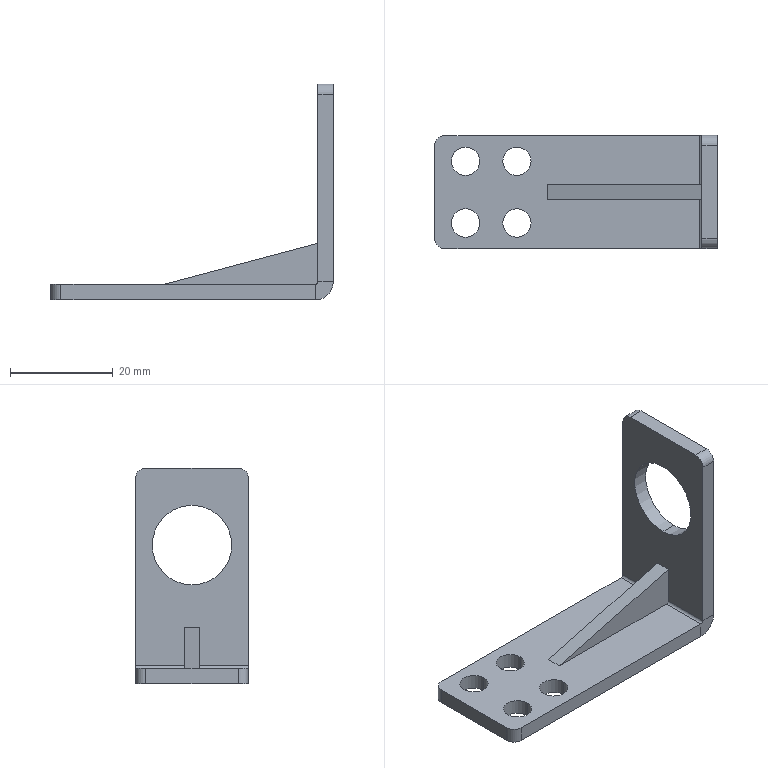Part | SolidWorks | features EdgeFlange 1, Fillet 1, FlatPattern 1, Gusset 1, HoleWzd 1, ICE 1, LPattern 1, SMBaseFlange 1, SheetMetal 1 | 2 solids | 33 faces | box 55 x 22 x 42 mm | volume 5646 mm3 | plane 17 | cylinder 16 | commonest cylinder face diameters 5.5 x8 4 x4 15.5 x2 1 x1 7 x1
STEP:
#1=CARTESIAN_POINT('',(24.5,1.5,8.));
#2=VERTEX_POINT('',#1);
#3=CARTESIAN_POINT('',(-5.5,1.5,0.));
#4=VERTEX_POINT('',#3);
#5=CARTESIAN_POINT('',(24.5,1.5,8.));
#6=DIRECTION('',(-0.9662,0.,-0.2577));
#7=VECTOR('',#6,1000.);
#8=LINE('',#5,#7);
#9=EDGE_CURVE('',#2,#4,#8,.T.);
#10=ORIENTED_EDGE('',*,*,#9,.T.);
#11=CARTESIAN_POINT('',(-5.5,-1.5,0.));
#12=VERTEX_POINT('',#11);
#13=CARTESIAN_POINT('',(-5.5,-1.5,0.));
#14=DIRECTION('',(0.,1.,0.));
#15=VECTOR('',#14,1000.);
#16=LINE('',#13,#15);
#17=EDGE_CURVE('',#12,#4,#16,.T.);
#18=ORIENTED_EDGE('',*,*,#17,.F.);
#19=CARTESIAN_POINT('',(24.5,-1.5,8.));
#20=VERTEX_POINT('',#19);
#21=CARTESIAN_POINT('',(24.5,-1.5,8.));
#22=DIRECTION('',(-0.9662,0.,-0.2577));
#23=VECTOR('',#22,1000.);
#24=LINE('',#21,#23);
#25=EDGE_CURVE('',#20,#12,#24,.T.);
#26=ORIENTED_EDGE('',*,*,#25,.F.);
#27=CARTESIAN_POINT('',(24.5,-1.5,8.));
#28=DIRECTION('',(0.,1.,0.));
#29=VECTOR('',#28,1000.);
#30=LINE('',#27,#29);
#31=EDGE_CURVE('',#20,#2,#30,.T.);
#32=ORIENTED_EDGE('',*,*,#31,.T.);
#33=EDGE_LOOP('',(#10,#18,#26,#32));
#34=FACE_OUTER_BOUND('',#33,.T.);
#35=CARTESIAN_POINT('',(24.5,-1.5,8.));
#36=DIRECTION('',(0.2577,0.,-0.9662));
#37=DIRECTION('',(-0.9662,0.,-0.2577));
#38=AXIS2_PLACEMENT_3D('',#35,#36,#37);
#39=PLANE('',#38);
#40=ADVANCED_FACE('',(#34),#39,.F.);
#41=CARTESIAN_POINT('',(24.5,1.5,0.));
#42=VERTEX_POINT('',#41);
#43=CARTESIAN_POINT('',(24.5,1.5,0.));
#44=DIRECTION('',(1.,0.,0.));
#45=VECTOR('',#44,1000.);
#46=LINE('',#43,#45);
#47=EDGE_CURVE('',#4,#42,#46,.T.);
#48=ORIENTED_EDGE('',*,*,#47,.T.);
#49=CARTESIAN_POINT('',(24.5,-1.5,0.));
#50=VERTEX_POINT('',#49);
#51=CARTESIAN_POINT('',(24.5,-1.5,0.));
#52=DIRECTION('',(0.,1.,0.));
#53=VECTOR('',#52,1000.);
#54=LINE('',#51,#53);
#55=EDGE_CURVE('',#50,#42,#54,.T.);
#56=ORIENTED_EDGE('',*,*,#55,.F.);
#57=CARTESIAN_POINT('',(24.5,-1.5,0.));
#58=DIRECTION('',(1.,0.,0.));
#59=VECTOR('',#58,1000.);
#60=LINE('',#57,#59);
#61=EDGE_CURVE('',#12,#50,#60,.T.);
#62=ORIENTED_EDGE('',*,*,#61,.F.);
#63=ORIENTED_EDGE('',*,*,#17,.T.);
#64=EDGE_LOOP('',(#48,#56,#62,#63));
#65=FACE_OUTER_BOUND('',#64,.T.);
#66=CARTESIAN_POINT('',(24.5,-1.5,0.));
#67=DIRECTION('',(0.,0.,1.));
#68=DIRECTION('',(1.,0.,0.));
#69=AXIS2_PLACEMENT_3D('',#66,#67,#68);
#70=PLANE('',#69);
#71=ADVANCED_FACE('',(#65),#70,.F.);
#72=CARTESIAN_POINT('',(24.5,1.5,0.));
#73=DIRECTION('',(0.,0.,1.));
#74=VECTOR('',#73,1000.);
#75=LINE('',#72,#74);
#76=EDGE_CURVE('',#42,#2,#75,.T.);
#77=ORIENTED_EDGE('',*,*,#76,.T.);
#78=ORIENTED_EDGE('',*,*,#31,.F.);
#79=CARTESIAN_POINT('',(24.5,-1.5,0.));
#80=DIRECTION('',(0.,0.,1.));
#81=VECTOR('',#80,1000.);
#82=LINE('',#79,#81);
#83=EDGE_CURVE('',#50,#20,#82,.T.);
#84=ORIENTED_EDGE('',*,*,#83,.F.);
#85=ORIENTED_EDGE('',*,*,#55,.T.);
#86=EDGE_LOOP('',(#77,#78,#84,#85));
#87=FACE_OUTER_BOUND('',#86,.T.);
#88=CARTESIAN_POINT('',(24.5,-1.5,0.));
#89=DIRECTION('',(-1.,0.,0.));
#90=DIRECTION('',(0.,0.,1.));
#91=AXIS2_PLACEMENT_3D('',#88,#89,#90);
#92=PLANE('',#91);
#93=ADVANCED_FACE('',(#87),#92,.F.);
#94=ORIENTED_EDGE('',*,*,#25,.T.);
#95=ORIENTED_EDGE('',*,*,#61,.T.);
#96=ORIENTED_EDGE('',*,*,#83,.T.);
#97=EDGE_LOOP('',(#94,#95,#96));
#98=FACE_OUTER_BOUND('',#97,.T.);
#99=CARTESIAN_POINT('',(0.,-1.5,0.));
#100=DIRECTION('',(0.,1.,0.));
#101=DIRECTION('',(0.,0.,1.));
#102=AXIS2_PLACEMENT_3D('',#99,#100,#101);
#103=PLANE('',#102);
#104=ADVANCED_FACE('',(#98),#103,.F.);
#105=ORIENTED_EDGE('',*,*,#9,.F.);
#106=ORIENTED_EDGE('',*,*,#76,.F.);
#107=ORIENTED_EDGE('',*,*,#47,.F.);
#108=EDGE_LOOP('',(#105,#106,#107));
#109=FACE_OUTER_BOUND('',#108,.T.);
#110=CARTESIAN_POINT('',(0.,1.5,0.));
#111=DIRECTION('',(0.,1.,0.));
#112=DIRECTION('',(0.,0.,1.));
#113=AXIS2_PLACEMENT_3D('',#110,#111,#112);
#114=PLANE('',#113);
#115=ADVANCED_FACE('',(#109),#114,.T.);
#116=CLOSED_SHELL('',(#40,#71,#93,#104,#115));
#117=MANIFOLD_SOLID_BREP('',#116);
#118=CARTESIAN_POINT('',(-14.25,6.,-3.));
#119=VERTEX_POINT('',#118);
#120=CARTESIAN_POINT('',(-8.75,6.,-3.));
#121=VERTEX_POINT('',#120);
#122=CARTESIAN_POINT('',(-11.5,6.,-3.));
#123=DIRECTION('',(0.,0.,1.));
#124=DIRECTION('',(1.,0.,0.));
#125=AXIS2_PLACEMENT_3D('',#122,#123,#124);
#126=CIRCLE('',#125,2.75);
#127=EDGE_CURVE('',#119,#121,#126,.T.);
#128=ORIENTED_EDGE('',*,*,#127,.F.);
#129=CARTESIAN_POINT('',(-14.25,6.,0.));
#130=VERTEX_POINT('',#129);
#131=CARTESIAN_POINT('',(-14.25,6.,0.));
#132=DIRECTION('',(0.,0.,1.));
#133=VECTOR('',#132,1000.);
#134=LINE('',#131,#133);
#135=EDGE_CURVE('',#119,#130,#134,.T.);
#136=ORIENTED_EDGE('',*,*,#135,.T.);
#137=CARTESIAN_POINT('',(-8.75,6.,0.));
#138=VERTEX_POINT('',#137);
#139=CARTESIAN_POINT('',(-11.5,6.,0.));
#140=DIRECTION('',(0.,0.,1.));
#141=DIRECTION('',(1.,0.,0.));
#142=AXIS2_PLACEMENT_3D('',#139,#140,#141);
#143=CIRCLE('',#142,2.75);
#144=EDGE_CURVE('',#130,#138,#143,.T.);
#145=ORIENTED_EDGE('',*,*,#144,.T.);
#146=CARTESIAN_POINT('',(-8.75,6.,0.));
#147=DIRECTION('',(0.,0.,1.));
#148=VECTOR('',#147,1000.);
#149=LINE('',#146,#148);
#150=EDGE_CURVE('',#121,#138,#149,.T.);
#151=ORIENTED_EDGE('',*,*,#150,.F.);
#152=EDGE_LOOP('',(#128,#136,#145,#151));
#153=FACE_OUTER_BOUND('',#152,.T.);
#154=CARTESIAN_POINT('',(-11.5,6.,0.));
#155=DIRECTION('',(0.,0.,1.));
#156=DIRECTION('',(1.,0.,0.));
#157=AXIS2_PLACEMENT_3D('',#154,#155,#156);
#158=CYLINDRICAL_SURFACE('',#157,2.75);
#159=ADVANCED_FACE('',(#153),#158,.F.);
#160=CARTESIAN_POINT('',(-14.25,-6.,-3.));
#161=VERTEX_POINT('',#160);
#162=CARTESIAN_POINT('',(-8.75,-6.,-3.));
#163=VERTEX_POINT('',#162);
#164=CARTESIAN_POINT('',(-11.5,-6.,-3.));
#165=DIRECTION('',(0.,0.,1.));
#166=DIRECTION('',(1.,0.,0.));
#167=AXIS2_PLACEMENT_3D('',#164,#165,#166);
#168=CIRCLE('',#167,2.75);
#169=EDGE_CURVE('',#161,#163,#168,.T.);
#170=ORIENTED_EDGE('',*,*,#169,.F.);
#171=CARTESIAN_POINT('',(-14.25,-6.,0.));
#172=VERTEX_POINT('',#171);
#173=CARTESIAN_POINT('',(-14.25,-6.,0.));
#174=DIRECTION('',(0.,0.,1.));
#175=VECTOR('',#174,1000.);
#176=LINE('',#173,#175);
#177=EDGE_CURVE('',#161,#172,#176,.T.);
#178=ORIENTED_EDGE('',*,*,#177,.T.);
#179=CARTESIAN_POINT('',(-8.75,-6.,0.));
#180=VERTEX_POINT('',#179);
#181=CARTESIAN_POINT('',(-11.5,-6.,0.));
#182=DIRECTION('',(0.,0.,1.));
#183=DIRECTION('',(1.,0.,0.));
#184=AXIS2_PLACEMENT_3D('',#181,#182,#183);
#185=CIRCLE('',#184,2.75);
#186=EDGE_CURVE('',#172,#180,#185,.T.);
#187=ORIENTED_EDGE('',*,*,#186,.T.);
#188=CARTESIAN_POINT('',(-8.75,-6.,0.));
#189=DIRECTION('',(0.,0.,1.));
#190=VECTOR('',#189,1000.);
#191=LINE('',#188,#190);
#192=EDGE_CURVE('',#163,#180,#191,.T.);
#193=ORIENTED_EDGE('',*,*,#192,.F.);
#194=EDGE_LOOP('',(#170,#178,#187,#193));
#195=FACE_OUTER_BOUND('',#194,.T.);
#196=CARTESIAN_POINT('',(-11.5,-6.,0.));
#197=DIRECTION('',(0.,0.,1.));
#198=DIRECTION('',(1.,0.,0.));
#199=AXIS2_PLACEMENT_3D('',#196,#197,#198);
#200=CYLINDRICAL_SURFACE('',#199,2.75);
#201=ADVANCED_FACE('',(#195),#200,.F.);
#202=CARTESIAN_POINT('',(-24.25,-6.,-3.));
#203=VERTEX_POINT('',#202);
#204=CARTESIAN_POINT('',(-18.75,-6.,-3.));
#205=VERTEX_POINT('',#204);
#206=CARTESIAN_POINT('',(-21.5,-6.,-3.));
#207=DIRECTION('',(0.,0.,1.));
#208=DIRECTION('',(1.,0.,0.));
#209=AXIS2_PLACEMENT_3D('',#206,#207,#208);
#210=CIRCLE('',#209,2.75);
#211=EDGE_CURVE('',#203,#205,#210,.T.);
#212=ORIENTED_EDGE('',*,*,#211,.F.);
#213=CARTESIAN_POINT('',(-24.25,-6.,0.));
#214=VERTEX_POINT('',#213);
#215=CARTESIAN_POINT('',(-24.25,-6.,0.));
#216=DIRECTION('',(0.,0.,1.));
#217=VECTOR('',#216,1000.);
#218=LINE('',#215,#217);
#219=EDGE_CURVE('',#203,#214,#218,.T.);
#220=ORIENTED_EDGE('',*,*,#219,.T.);
#221=CARTESIAN_POINT('',(-18.75,-6.,0.));
#222=VERTEX_POINT('',#221);
#223=CARTESIAN_POINT('',(-21.5,-6.,0.));
#224=DIRECTION('',(0.,0.,1.));
#225=DIRECTION('',(1.,0.,0.));
#226=AXIS2_PLACEMENT_3D('',#223,#224,#225);
#227=CIRCLE('',#226,2.75);
#228=EDGE_CURVE('',#214,#222,#227,.T.);
#229=ORIENTED_EDGE('',*,*,#228,.T.);
#230=CARTESIAN_POINT('',(-18.75,-6.,0.));
#231=DIRECTION('',(0.,0.,1.));
#232=VECTOR('',#231,1000.);
#233=LINE('',#230,#232);
#234=EDGE_CURVE('',#205,#222,#233,.T.);
#235=ORIENTED_EDGE('',*,*,#234,.F.);
#236=EDGE_LOOP('',(#212,#220,#229,#235));
#237=FACE_OUTER_BOUND('',#236,.T.);
#238=CARTESIAN_POINT('',(-21.5,-6.,0.));
#239=DIRECTION('',(0.,0.,1.));
#240=DIRECTION('',(1.,0.,0.));
#241=AXIS2_PLACEMENT_3D('',#238,#239,#240);
#242=CYLINDRICAL_SURFACE('',#241,2.75);
#243=ADVANCED_FACE('',(#237),#242,.F.);
#244=CARTESIAN_POINT('',(-24.25,6.,-3.));
#245=VERTEX_POINT('',#244);
#246=CARTESIAN_POINT('',(-18.75,6.,-3.));
#247=VERTEX_POINT('',#246);
#248=CARTESIAN_POINT('',(-21.5,6.,-3.));
#249=DIRECTION('',(0.,0.,1.));
#250=DIRECTION('',(1.,0.,0.));
#251=AXIS2_PLACEMENT_3D('',#248,#249,#250);
#252=CIRCLE('',#251,2.75);
#253=EDGE_CURVE('',#245,#247,#252,.T.);
#254=ORIENTED_EDGE('',*,*,#253,.F.);
#255=CARTESIAN_POINT('',(-24.25,6.,0.));
#256=VERTEX_POINT('',#255);
#257=CARTESIAN_POINT('',(-24.25,6.,0.));
#258=DIRECTION('',(0.,0.,1.));
#259=VECTOR('',#258,1000.);
#260=LINE('',#257,#259);
#261=EDGE_CURVE('',#245,#256,#260,.T.);
#262=ORIENTED_EDGE('',*,*,#261,.T.);
#263=CARTESIAN_POINT('',(-18.75,6.,0.));
#264=VERTEX_POINT('',#263);
#265=CARTESIAN_POINT('',(-21.5,6.,0.));
#266=DIRECTION('',(0.,0.,1.));
#267=DIRECTION('',(1.,0.,0.));
#268=AXIS2_PLACEMENT_3D('',#265,#266,#267);
#269=CIRCLE('',#268,2.75);
#270=EDGE_CURVE('',#256,#264,#269,.T.);
#271=ORIENTED_EDGE('',*,*,#270,.T.);
#272=CARTESIAN_POINT('',(-18.75,6.,0.));
#273=DIRECTION('',(0.,0.,1.));
#274=VECTOR('',#273,1000.);
#275=LINE('',#272,#274);
#276=EDGE_CURVE('',#247,#264,#275,.T.);
#277=ORIENTED_EDGE('',*,*,#276,.F.);
#278=EDGE_LOOP('',(#254,#262,#271,#277));
#279=FACE_OUTER_BOUND('',#278,.T.);
#280=CARTESIAN_POINT('',(-21.5,6.,0.));
#281=DIRECTION('',(0.,0.,1.));
#282=DIRECTION('',(1.,0.,0.));
#283=AXIS2_PLACEMENT_3D('',#280,#281,#282);
#284=CYLINDRICAL_SURFACE('',#283,2.75);
#285=ADVANCED_FACE('',(#279),#284,.F.);
#286=CARTESIAN_POINT('',(27.5,0.,31.75));
#287=VERTEX_POINT('',#286);
#288=CARTESIAN_POINT('',(27.5,0.,16.25));
#289=VERTEX_POINT('',#288);
#290=CARTESIAN_POINT('',(27.5,0.,24.));
#291=DIRECTION('',(1.,0.,0.));
#292=DIRECTION('',(0.,0.,1.));
#293=AXIS2_PLACEMENT_3D('',#290,#291,#292);
#294=CIRCLE('',#293,7.75);
#295=EDGE_CURVE('',#287,#289,#294,.T.);
#296=ORIENTED_EDGE('',*,*,#295,.T.);
#297=CARTESIAN_POINT('',(24.5,0.,16.25));
#298=VERTEX_POINT('',#297);
#299=CARTESIAN_POINT('',(27.501,0.,16.25));
#300=DIRECTION('',(-1.,0.,0.));
#301=VECTOR('',#300,1000.);
#302=LINE('',#299,#301);
#303=EDGE_CURVE('',#289,#298,#302,.T.);
#304=ORIENTED_EDGE('',*,*,#303,.T.);
#305=CARTESIAN_POINT('',(24.5,0.,31.75));
#306=VERTEX_POINT('',#305);
#307=CARTESIAN_POINT('',(24.5,0.,24.));
#308=DIRECTION('',(-1.,0.,0.));
#309=DIRECTION('',(0.,0.,1.));
#310=AXIS2_PLACEMENT_3D('',#307,#308,#309);
#311=CIRCLE('',#310,7.75);
#312=EDGE_CURVE('',#298,#306,#311,.T.);
#313=ORIENTED_EDGE('',*,*,#312,.T.);
#314=CARTESIAN_POINT('',(27.501,0.,31.75));
#315=DIRECTION('',(-1.,0.,0.));
#316=VECTOR('',#315,1000.);
#317=LINE('',#314,#316);
#318=EDGE_CURVE('',#287,#306,#317,.T.);
#319=ORIENTED_EDGE('',*,*,#318,.F.);
#320=EDGE_LOOP('',(#296,#304,#313,#319));
#321=FACE_OUTER_BOUND('',#320,.T.);
#322=CARTESIAN_POINT('',(27.501,0.,24.));
#323=DIRECTION('',(-1.,0.,0.));
#324=DIRECTION('',(0.,0.,1.));
#325=AXIS2_PLACEMENT_3D('',#322,#323,#324);
#326=CYLINDRICAL_SURFACE('',#325,7.75);
#327=ADVANCED_FACE('',(#321),#326,.F.);
#328=CARTESIAN_POINT('',(24.,11.,-3.));
#329=VERTEX_POINT('',#328);
#330=CARTESIAN_POINT('',(-25.5,11.,-3.));
#331=VERTEX_POINT('',#330);
#332=CARTESIAN_POINT('',(27.5,11.,-3.));
#333=DIRECTION('',(-1.,0.,0.));
#334=VECTOR('',#333,1000.);
#335=LINE('',#332,#334);
#336=EDGE_CURVE('',#329,#331,#335,.T.);
#337=ORIENTED_EDGE('',*,*,#336,.T.);
#338=CARTESIAN_POINT('',(-25.5,11.,0.));
#339=VERTEX_POINT('',#338);
#340=CARTESIAN_POINT('',(-25.5,11.,-3.));
#341=DIRECTION('',(0.,0.,1.));
#342=VECTOR('',#341,1000.);
#343=LINE('',#340,#342);
#344=EDGE_CURVE('',#331,#339,#343,.T.);
#345=ORIENTED_EDGE('',*,*,#344,.T.);
#346=CARTESIAN_POINT('',(24.,11.,0.));
#347=VERTEX_POINT('',#346);
#348=CARTESIAN_POINT('',(27.5,11.,0.));
#349=DIRECTION('',(-1.,0.,0.));
#350=VECTOR('',#349,1000.);
#351=LINE('',#348,#350);
#352=EDGE_CURVE('',#347,#339,#351,.T.);
#353=ORIENTED_EDGE('',*,*,#352,.F.);
#354=CARTESIAN_POINT('',(24.,11.,0.));
#355=DIRECTION('',(0.,0.,-1.));
#356=VECTOR('',#355,1000.);
#357=LINE('',#354,#356);
#358=EDGE_CURVE('',#347,#329,#357,.T.);
#359=ORIENTED_EDGE('',*,*,#358,.T.);
#360=EDGE_LOOP('',(#337,#345,#353,#359));
#361=FACE_OUTER_BOUND('',#360,.T.);
#362=CARTESIAN_POINT('',(27.5,11.,-3.));
#363=DIRECTION('',(0.,1.,0.));
#364=DIRECTION('',(-1.,0.,0.));
#365=AXIS2_PLACEMENT_3D('',#362,#363,#364);
#366=PLANE('',#365);
#367=ADVANCED_FACE('',(#361),#366,.T.);
#368=CARTESIAN_POINT('',(-11.5,6.,-3.));
#369=DIRECTION('',(0.,0.,1.));
#370=DIRECTION('',(1.,0.,0.));
#371=AXIS2_PLACEMENT_3D('',#368,#369,#370);
#372=CIRCLE('',#371,2.75);
#373=EDGE_CURVE('',#121,#119,#372,.T.);
#374=ORIENTED_EDGE('',*,*,#373,.T.);
#375=ORIENTED_EDGE('',*,*,#127,.T.);
#376=EDGE_LOOP('',(#374,#375));
#377=FACE_BOUND('',#376,.T.);
#378=CARTESIAN_POINT('',(-11.5,-6.,-3.));
#379=DIRECTION('',(0.,0.,1.));
#380=DIRECTION('',(1.,0.,0.));
#381=AXIS2_PLACEMENT_3D('',#378,#379,#380);
#382=CIRCLE('',#381,2.75);
#383=EDGE_CURVE('',#163,#161,#382,.T.);
#384=ORIENTED_EDGE('',*,*,#383,.T.);
#385=ORIENTED_EDGE('',*,*,#169,.T.);
#386=EDGE_LOOP('',(#384,#385));
#387=FACE_BOUND('',#386,.T.);
#388=CARTESIAN_POINT('',(-21.5,-6.,-3.));
#389=DIRECTION('',(0.,0.,1.));
#390=DIRECTION('',(1.,0.,0.));
#391=AXIS2_PLACEMENT_3D('',#388,#389,#390);
#392=CIRCLE('',#391,2.75);
#393=EDGE_CURVE('',#205,#203,#392,.T.);
#394=ORIENTED_EDGE('',*,*,#393,.T.);
#395=ORIENTED_EDGE('',*,*,#211,.T.);
#396=EDGE_LOOP('',(#394,#395));
#397=FACE_BOUND('',#396,.T.);
#398=CARTESIAN_POINT('',(-21.5,6.,-3.));
#399=DIRECTION('',(0.,0.,1.));
#400=DIRECTION('',(1.,0.,0.));
#401=AXIS2_PLACEMENT_3D('',#398,#399,#400);
#402=CIRCLE('',#401,2.75);
#403=EDGE_CURVE('',#247,#245,#402,.T.);
#404=ORIENTED_EDGE('',*,*,#403,.T.);
#405=ORIENTED_EDGE('',*,*,#253,.T.);
#406=EDGE_LOOP('',(#404,#405));
#407=FACE_BOUND('',#406,.T.);
#408=CARTESIAN_POINT('',(-27.5,9.,-3.));
#409=VERTEX_POINT('',#408);
#410=CARTESIAN_POINT('',(-27.5,-9.,-3.));
#411=VERTEX_POINT('',#410);
#412=CARTESIAN_POINT('',(-27.5,-11.,-3.));
#413=DIRECTION('',(0.,-1.,0.));
#414=VECTOR('',#413,1000.);
#415=LINE('',#412,#414);
#416=EDGE_CURVE('',#409,#411,#415,.T.);
#417=ORIENTED_EDGE('',*,*,#416,.F.);
#418=CARTESIAN_POINT('',(-25.5,9.,-3.));
#419=DIRECTION('',(0.,0.,-1.));
#420=DIRECTION('',(1.,0.,0.));
#421=AXIS2_PLACEMENT_3D('',#418,#419,#420);
#422=CIRCLE('',#421,2.);
#423=EDGE_CURVE('',#409,#331,#422,.T.);
#424=ORIENTED_EDGE('',*,*,#423,.T.);
#425=ORIENTED_EDGE('',*,*,#336,.F.);
#426=CARTESIAN_POINT('',(24.,-11.,-3.));
#427=VERTEX_POINT('',#426);
#428=CARTESIAN_POINT('',(24.,11.,-3.));
#429=DIRECTION('',(0.,-1.,0.));
#430=VECTOR('',#429,1000.);
#431=LINE('',#428,#430);
#432=EDGE_CURVE('',#329,#427,#431,.T.);
#433=ORIENTED_EDGE('',*,*,#432,.T.);
#434=CARTESIAN_POINT('',(-25.5,-11.,-3.));
#435=VERTEX_POINT('',#434);
#436=CARTESIAN_POINT('',(27.5,-11.,-3.));
#437=DIRECTION('',(1.,0.,0.));
#438=VECTOR('',#437,1000.);
#439=LINE('',#436,#438);
#440=EDGE_CURVE('',#435,#427,#439,.T.);
#441=ORIENTED_EDGE('',*,*,#440,.F.);
#442=CARTESIAN_POINT('',(-25.5,-9.,-3.));
#443=DIRECTION('',(0.,0.,-1.));
#444=DIRECTION('',(1.,0.,0.));
#445=AXIS2_PLACEMENT_3D('',#442,#443,#444);
#446=CIRCLE('',#445,2.);
#447=EDGE_CURVE('',#435,#411,#446,.T.);
#448=ORIENTED_EDGE('',*,*,#447,.T.);
#449=EDGE_LOOP('',(#417,#424,#425,#433,#441,#448));
#450=FACE_OUTER_BOUND('',#449,.T.);
#451=CARTESIAN_POINT('',(0.,0.,-3.));
#452=DIRECTION('',(0.,0.,1.));
#453=DIRECTION('',(1.,0.,0.));
#454=AXIS2_PLACEMENT_3D('',#451,#452,#453);
#455=PLANE('',#454);
#456=ADVANCED_FACE('',(#377,#387,#397,#407,#450),#455,.F.);
#457=CARTESIAN_POINT('',(-11.5,6.,0.));
#458=DIRECTION('',(0.,0.,1.));
#459=DIRECTION('',(1.,0.,0.));
#460=AXIS2_PLACEMENT_3D('',#457,#458,#459);
#461=CIRCLE('',#460,2.75);
#462=EDGE_CURVE('',#138,#130,#461,.T.);
#463=ORIENTED_EDGE('',*,*,#462,.F.);
#464=ORIENTED_EDGE('',*,*,#144,.F.);
#465=EDGE_LOOP('',(#463,#464));
#466=FACE_BOUND('',#465,.T.);
#467=CARTESIAN_POINT('',(-11.5,-6.,0.));
#468=DIRECTION('',(0.,0.,1.));
#469=DIRECTION('',(1.,0.,0.));
#470=AXIS2_PLACEMENT_3D('',#467,#468,#469);
#471=CIRCLE('',#470,2.75);
#472=EDGE_CURVE('',#180,#172,#471,.T.);
#473=ORIENTED_EDGE('',*,*,#472,.F.);
#474=ORIENTED_EDGE('',*,*,#186,.F.);
#475=EDGE_LOOP('',(#473,#474));
#476=FACE_BOUND('',#475,.T.);
#477=CARTESIAN_POINT('',(-21.5,-6.,0.));
#478=DIRECTION('',(0.,0.,1.));
#479=DIRECTION('',(1.,0.,0.));
#480=AXIS2_PLACEMENT_3D('',#477,#478,#479);
#481=CIRCLE('',#480,2.75);
#482=EDGE_CURVE('',#222,#214,#481,.T.);
#483=ORIENTED_EDGE('',*,*,#482,.F.);
#484=ORIENTED_EDGE('',*,*,#228,.F.);
#485=EDGE_LOOP('',(#483,#484));
#486=FACE_BOUND('',#485,.T.);
#487=CARTESIAN_POINT('',(-21.5,6.,0.));
#488=DIRECTION('',(0.,0.,1.));
#489=DIRECTION('',(1.,0.,0.));
#490=AXIS2_PLACEMENT_3D('',#487,#488,#489);
#491=CIRCLE('',#490,2.75);
#492=EDGE_CURVE('',#264,#256,#491,.T.);
#493=ORIENTED_EDGE('',*,*,#492,.F.);
#494=ORIENTED_EDGE('',*,*,#270,.F.);
#495=EDGE_LOOP('',(#493,#494));
#496=FACE_BOUND('',#495,.T.);
#497=ORIENTED_EDGE('',*,*,#352,.T.);
#498=CARTESIAN_POINT('',(-27.5,9.,0.));
#499=VERTEX_POINT('',#498);
#500=CARTESIAN_POINT('',(-25.5,9.,0.));
#501=DIRECTION('',(0.,0.,1.));
#502=DIRECTION('',(1.,0.,0.));
#503=AXIS2_PLACEMENT_3D('',#500,#501,#502);
#504=CIRCLE('',#503,2.);
#505=EDGE_CURVE('',#339,#499,#504,.T.);
#506=ORIENTED_EDGE('',*,*,#505,.T.);
#507=CARTESIAN_POINT('',(-27.5,-9.,0.));
#508=VERTEX_POINT('',#507);
#509=CARTESIAN_POINT('',(-27.5,-11.,0.));
#510=DIRECTION('',(0.,-1.,0.));
#511=VECTOR('',#510,1000.);
#512=LINE('',#509,#511);
#513=EDGE_CURVE('',#499,#508,#512,.T.);
#514=ORIENTED_EDGE('',*,*,#513,.T.);
#515=CARTESIAN_POINT('',(-25.5,-11.,0.));
#516=VERTEX_POINT('',#515);
#517=CARTESIAN_POINT('',(-25.5,-9.,0.));
#518=DIRECTION('',(0.,0.,1.));
#519=DIRECTION('',(1.,0.,0.));
#520=AXIS2_PLACEMENT_3D('',#517,#518,#519);
#521=CIRCLE('',#520,2.);
#522=EDGE_CURVE('',#508,#516,#521,.T.);
#523=ORIENTED_EDGE('',*,*,#522,.T.);
#524=CARTESIAN_POINT('',(24.,-11.,0.));
#525=VERTEX_POINT('',#524);
#526=CARTESIAN_POINT('',(27.5,-11.,0.));
#527=DIRECTION('',(1.,0.,0.));
#528=VECTOR('',#527,1000.);
#529=LINE('',#526,#528);
#530=EDGE_CURVE('',#516,#525,#529,.T.);
#531=ORIENTED_EDGE('',*,*,#530,.T.);
#532=CARTESIAN_POINT('',(24.,11.,0.));
#533=DIRECTION('',(0.,-1.,0.));
#534=VECTOR('',#533,1000.);
#535=LINE('',#532,#534);
#536=EDGE_CURVE('',#347,#525,#535,.T.);
#537=ORIENTED_EDGE('',*,*,#536,.F.);
#538=EDGE_LOOP('',(#497,#506,#514,#523,#531,#537));
#539=FACE_OUTER_BOUND('',#538,.T.);
#540=CARTESIAN_POINT('',(0.,0.,0.));
#541=DIRECTION('',(0.,0.,1.));
#542=DIRECTION('',(1.,0.,0.));
#543=AXIS2_PLACEMENT_3D('',#540,#541,#542);
#544=PLANE('',#543);
#545=ADVANCED_FACE('',(#466,#476,#486,#496,#539),#544,.T.);
#546=ORIENTED_EDGE('',*,*,#513,.F.);
#547=CARTESIAN_POINT('',(-27.5,9.,-3.));
#548=DIRECTION('',(0.,0.,-1.));
#549=VECTOR('',#548,1000.);
#550=LINE('',#547,#549);
#551=EDGE_CURVE('',#499,#409,#550,.T.);
#552=ORIENTED_EDGE('',*,*,#551,.T.);
#553=ORIENTED_EDGE('',*,*,#416,.T.);
#554=CARTESIAN_POINT('',(-27.5,-9.,-3.));
#555=DIRECTION('',(0.,0.,1.));
#556=VECTOR('',#555,1000.);
#557=LINE('',#554,#556);
#558=EDGE_CURVE('',#411,#508,#557,.T.);
#559=ORIENTED_EDGE('',*,*,#558,.T.);
#560=EDGE_LOOP('',(#546,#552,#553,#559));
#561=FACE_OUTER_BOUND('',#560,.T.);
#562=CARTESIAN_POINT('',(-27.5,-11.,-3.));
#563=DIRECTION('',(-1.,0.,0.));
#564=DIRECTION('',(0.,0.,1.));
#565=AXIS2_PLACEMENT_3D('',#562,#563,#564);
#566=PLANE('',#565);
#567=ADVANCED_FACE('',(#561),#566,.T.);
#568=ORIENTED_EDGE('',*,*,#530,.F.);
#569=CARTESIAN_POINT('',(-25.5,-11.,-3.));
#570=DIRECTION('',(0.,0.,-1.));
#571=VECTOR('',#570,1000.);
#572=LINE('',#569,#571);
#573=EDGE_CURVE('',#516,#435,#572,.T.);
#574=ORIENTED_EDGE('',*,*,#573,.T.);
#575=ORIENTED_EDGE('',*,*,#440,.T.);
#576=CARTESIAN_POINT('',(24.,-11.,0.));
#577=DIRECTION('',(0.,0.,-1.));
#578=VECTOR('',#577,1000.);
#579=LINE('',#576,#578);
#580=EDGE_CURVE('',#525,#427,#579,.T.);
#581=ORIENTED_EDGE('',*,*,#580,.F.);
#582=EDGE_LOOP('',(#568,#574,#575,#581));
#583=FACE_OUTER_BOUND('',#582,.T.);
#584=CARTESIAN_POINT('',(27.5,-11.,-3.));
#585=DIRECTION('',(0.,-1.,0.));
#586=DIRECTION('',(1.,0.,0.));
#587=AXIS2_PLACEMENT_3D('',#584,#585,#586);
#588=PLANE('',#587);
#589=ADVANCED_FACE('',(#583),#588,.T.);
#590=CARTESIAN_POINT('',(24.5,-11.,0.5));
#591=VERTEX_POINT('',#590);
#592=CARTESIAN_POINT('',(27.5,-11.,0.5));
#593=VERTEX_POINT('',#592);
#594=CARTESIAN_POINT('',(27.5,-11.,0.5));
#595=DIRECTION('',(1.,0.,0.));
#596=VECTOR('',#595,1000.);
#597=LINE('',#594,#596);
#598=EDGE_CURVE('',#591,#593,#597,.T.);
#599=ORIENTED_EDGE('',*,*,#598,.F.);
#600=CARTESIAN_POINT('',(24.,-11.,0.5));
#601=DIRECTION('',(0.,-1.,0.));
#602=DIRECTION('',(0.,0.,1.));
#603=AXIS2_PLACEMENT_3D('',#600,#601,#602);
#604=CIRCLE('',#603,0.5);
#605=EDGE_CURVE('',#525,#591,#604,.T.);
#606=ORIENTED_EDGE('',*,*,#605,.F.);
#607=ORIENTED_EDGE('',*,*,#580,.T.);
#608=CARTESIAN_POINT('',(24.,-11.,0.5));
#609=DIRECTION('',(0.,-1.,0.));
#610=DIRECTION('',(0.,0.,1.));
#611=AXIS2_PLACEMENT_3D('',#608,#609,#610);
#612=CIRCLE('',#611,3.5);
#613=EDGE_CURVE('',#427,#593,#612,.T.);
#614=ORIENTED_EDGE('',*,*,#613,.T.);
#615=EDGE_LOOP('',(#599,#606,#607,#614));
#616=FACE_OUTER_BOUND('',#615,.T.);
#617=CARTESIAN_POINT('',(24.,-11.,0.5));
#618=DIRECTION('',(0.,-1.,0.));
#619=DIRECTION('',(0.,0.,-1.));
#620=AXIS2_PLACEMENT_3D('',#617,#618,#619);
#621=PLANE('',#620);
#622=ADVANCED_FACE('',(#616),#621,.T.);
#623=CARTESIAN_POINT('',(24.5,11.,0.5));
#624=VERTEX_POINT('',#623);
#625=CARTESIAN_POINT('',(24.,11.,0.5));
#626=DIRECTION('',(0.,1.,0.));
#627=DIRECTION('',(0.,0.,1.));
#628=AXIS2_PLACEMENT_3D('',#625,#626,#627);
#629=CIRCLE('',#628,0.5);
#630=EDGE_CURVE('',#624,#347,#629,.T.);
#631=ORIENTED_EDGE('',*,*,#630,.F.);
#632=CARTESIAN_POINT('',(27.5,11.,0.5));
#633=VERTEX_POINT('',#632);
#634=CARTESIAN_POINT('',(24.5,11.,0.5));
#635=DIRECTION('',(1.,0.,0.));
#636=VECTOR('',#635,1000.);
#637=LINE('',#634,#636);
#638=EDGE_CURVE('',#624,#633,#637,.T.);
#639=ORIENTED_EDGE('',*,*,#638,.T.);
#640=CARTESIAN_POINT('',(24.,11.,0.5));
#641=DIRECTION('',(0.,1.,0.));
#642=DIRECTION('',(0.,0.,1.));
#643=AXIS2_PLACEMENT_3D('',#640,#641,#642);
#644=CIRCLE('',#643,3.5);
#645=EDGE_CURVE('',#633,#329,#644,.T.);
#646=ORIENTED_EDGE('',*,*,#645,.T.);
#647=ORIENTED_EDGE('',*,*,#358,.F.);
#648=EDGE_LOOP('',(#631,#639,#646,#647));
#649=FACE_OUTER_BOUND('',#648,.T.);
#650=CARTESIAN_POINT('',(24.,11.,0.5));
#651=DIRECTION('',(0.,-1.,0.));
#652=DIRECTION('',(0.,0.,-1.));
#653=AXIS2_PLACEMENT_3D('',#650,#651,#652);
#654=PLANE('',#653);
#655=ADVANCED_FACE('',(#649),#654,.F.);
#656=ORIENTED_EDGE('',*,*,#432,.F.);
#657=ORIENTED_EDGE('',*,*,#645,.F.);
#658=CARTESIAN_POINT('',(27.5,-11.,0.5));
#659=DIRECTION('',(0.,-1.,0.));
#660=VECTOR('',#659,1000.);
#661=LINE('',#658,#660);
#662=EDGE_CURVE('',#633,#593,#661,.T.);
#663=ORIENTED_EDGE('',*,*,#662,.T.);
#664=ORIENTED_EDGE('',*,*,#613,.F.);
#665=EDGE_LOOP('',(#656,#657,#663,#664));
#666=FACE_OUTER_BOUND('',#665,.T.);
#667=CARTESIAN_POINT('',(24.,11.,0.5));
#668=DIRECTION('',(0.,1.,0.));
#669=DIRECTION('',(1.,0.,0.));
#670=AXIS2_PLACEMENT_3D('',#667,#668,#669);
#671=CYLINDRICAL_SURFACE('',#670,3.5);
#672=ADVANCED_FACE('',(#666),#671,.T.);
#673=ORIENTED_EDGE('',*,*,#536,.T.);
#674=ORIENTED_EDGE('',*,*,#605,.T.);
#675=CARTESIAN_POINT('',(24.5,-11.,0.5));
#676=DIRECTION('',(0.,1.,0.));
#677=VECTOR('',#676,1000.);
#678=LINE('',#675,#677);
#679=EDGE_CURVE('',#591,#624,#678,.T.);
#680=ORIENTED_EDGE('',*,*,#679,.T.);
#681=ORIENTED_EDGE('',*,*,#630,.T.);
#682=EDGE_LOOP('',(#673,#674,#680,#681));
#683=FACE_OUTER_BOUND('',#682,.T.);
#684=CARTESIAN_POINT('',(24.,11.,0.5));
#685=DIRECTION('',(0.,1.,0.));
#686=DIRECTION('',(1.,0.,0.));
#687=AXIS2_PLACEMENT_3D('',#684,#685,#686);
#688=CYLINDRICAL_SURFACE('',#687,0.5);
#689=ADVANCED_FACE('',(#683),#688,.F.);
#690=CARTESIAN_POINT('',(27.5,-11.,37.));
#691=VERTEX_POINT('',#690);
#692=CARTESIAN_POINT('',(27.5,-11.,0.));
#693=DIRECTION('',(0.,0.,-1.));
#694=VECTOR('',#693,1000.);
#695=LINE('',#692,#694);
#696=EDGE_CURVE('',#691,#593,#695,.T.);
#697=ORIENTED_EDGE('',*,*,#696,.F.);
#698=CARTESIAN_POINT('',(24.5,-11.,37.));
#699=VERTEX_POINT('',#698);
#700=CARTESIAN_POINT('',(27.5,-11.,37.));
#701=DIRECTION('',(-1.,0.,0.));
#702=VECTOR('',#701,1000.);
#703=LINE('',#700,#702);
#704=EDGE_CURVE('',#691,#699,#703,.T.);
#705=ORIENTED_EDGE('',*,*,#704,.T.);
#706=CARTESIAN_POINT('',(24.5,-11.,0.));
#707=DIRECTION('',(0.,0.,-1.));
#708=VECTOR('',#707,1000.);
#709=LINE('',#706,#708);
#710=EDGE_CURVE('',#699,#591,#709,.T.);
#711=ORIENTED_EDGE('',*,*,#710,.T.);
#712=ORIENTED_EDGE('',*,*,#598,.T.);
#713=EDGE_LOOP('',(#697,#705,#711,#712));
#714=FACE_OUTER_BOUND('',#713,.T.);
#715=CARTESIAN_POINT('',(27.5,-11.,0.));
#716=DIRECTION('',(0.,1.,0.));
#717=DIRECTION('',(0.,0.,1.));
#718=AXIS2_PLACEMENT_3D('',#715,#716,#717);
#719=PLANE('',#718);
#720=ADVANCED_FACE('',(#714),#719,.F.);
#721=CARTESIAN_POINT('',(24.5,11.,37.));
#722=VERTEX_POINT('',#721);
#723=CARTESIAN_POINT('',(24.5,11.,39.));
#724=DIRECTION('',(0.,0.,1.));
#725=VECTOR('',#724,1000.);
#726=LINE('',#723,#725);
#727=EDGE_CURVE('',#624,#722,#726,.T.);
#728=ORIENTED_EDGE('',*,*,#727,.T.);
#729=CARTESIAN_POINT('',(27.5,11.,37.));
#730=VERTEX_POINT('',#729);
#731=CARTESIAN_POINT('',(27.5,11.,37.));
#732=DIRECTION('',(1.,0.,0.));
#733=VECTOR('',#732,1000.);
#734=LINE('',#731,#733);
#735=EDGE_CURVE('',#722,#730,#734,.T.);
#736=ORIENTED_EDGE('',*,*,#735,.T.);
#737=CARTESIAN_POINT('',(27.5,11.,0.));
#738=DIRECTION('',(0.,0.,1.));
#739=VECTOR('',#738,1000.);
#740=LINE('',#737,#739);
#741=EDGE_CURVE('',#633,#730,#740,.T.);
#742=ORIENTED_EDGE('',*,*,#741,.F.);
#743=ORIENTED_EDGE('',*,*,#638,.F.);
#744=EDGE_LOOP('',(#728,#736,#742,#743));
#745=FACE_OUTER_BOUND('',#744,.T.);
#746=CARTESIAN_POINT('',(27.5,11.,39.));
#747=DIRECTION('',(0.,-1.,0.));
#748=DIRECTION('',(0.,0.,-1.));
#749=AXIS2_PLACEMENT_3D('',#746,#747,#748);
#750=PLANE('',#749);
#751=ADVANCED_FACE('',(#745),#750,.F.);
#752=ORIENTED_EDGE('',*,*,#295,.F.);
#753=CARTESIAN_POINT('',(27.5,0.,24.));
#754=DIRECTION('',(1.,0.,0.));
#755=DIRECTION('',(0.,0.,1.));
#756=AXIS2_PLACEMENT_3D('',#753,#754,#755);
#757=CIRCLE('',#756,7.75);
#758=EDGE_CURVE('',#289,#287,#757,.T.);
#759=ORIENTED_EDGE('',*,*,#758,.F.);
#760=EDGE_LOOP('',(#752,#759));
#761=FACE_BOUND('',#760,.T.);
#762=ORIENTED_EDGE('',*,*,#741,.T.);
#763=CARTESIAN_POINT('',(27.5,9.,39.));
#764=VERTEX_POINT('',#763);
#765=CARTESIAN_POINT('',(27.5,9.,37.));
#766=DIRECTION('',(1.,0.,0.));
#767=DIRECTION('',(0.,0.,1.));
#768=AXIS2_PLACEMENT_3D('',#765,#766,#767);
#769=CIRCLE('',#768,2.);
#770=EDGE_CURVE('',#730,#764,#769,.T.);
#771=ORIENTED_EDGE('',*,*,#770,.T.);
#772=CARTESIAN_POINT('',(27.5,-9.,39.));
#773=VERTEX_POINT('',#772);
#774=CARTESIAN_POINT('',(27.5,0.,39.));
#775=DIRECTION('',(0.,-1.,0.));
#776=VECTOR('',#775,1000.);
#777=LINE('',#774,#776);
#778=EDGE_CURVE('',#764,#773,#777,.T.);
#779=ORIENTED_EDGE('',*,*,#778,.T.);
#780=CARTESIAN_POINT('',(27.5,-9.,37.));
#781=DIRECTION('',(1.,0.,0.));
#782=DIRECTION('',(0.,0.,1.));
#783=AXIS2_PLACEMENT_3D('',#780,#781,#782);
#784=CIRCLE('',#783,2.);
#785=EDGE_CURVE('',#773,#691,#784,.T.);
#786=ORIENTED_EDGE('',*,*,#785,.T.);
#787=ORIENTED_EDGE('',*,*,#696,.T.);
#788=ORIENTED_EDGE('',*,*,#662,.F.);
#789=EDGE_LOOP('',(#762,#771,#779,#786,#787,#788));
#790=FACE_OUTER_BOUND('',#789,.T.);
#791=CARTESIAN_POINT('',(27.5,0.,0.));
#792=DIRECTION('',(-1.,0.,0.));
#793=DIRECTION('',(0.,0.,1.));
#794=AXIS2_PLACEMENT_3D('',#791,#792,#793);
#795=PLANE('',#794);
#796=ADVANCED_FACE('',(#761,#790),#795,.F.);
#797=CARTESIAN_POINT('',(24.5,0.,24.));
#798=DIRECTION('',(-1.,0.,0.));
#799=DIRECTION('',(0.,0.,1.));
#800=AXIS2_PLACEMENT_3D('',#797,#798,#799);
#801=CIRCLE('',#800,7.75);
#802=EDGE_CURVE('',#306,#298,#801,.T.);
#803=ORIENTED_EDGE('',*,*,#802,.F.);
#804=ORIENTED_EDGE('',*,*,#312,.F.);
#805=EDGE_LOOP('',(#803,#804));
#806=FACE_BOUND('',#805,.T.);
#807=CARTESIAN_POINT('',(24.5,9.,39.));
#808=VERTEX_POINT('',#807);
#809=CARTESIAN_POINT('',(24.5,-9.,39.));
#810=VERTEX_POINT('',#809);
#811=CARTESIAN_POINT('',(24.5,-11.,39.));
#812=DIRECTION('',(0.,-1.,0.));
#813=VECTOR('',#812,1000.);
#814=LINE('',#811,#813);
#815=EDGE_CURVE('',#808,#810,#814,.T.);
#816=ORIENTED_EDGE('',*,*,#815,.F.);
#817=CARTESIAN_POINT('',(24.5,9.,37.));
#818=DIRECTION('',(-1.,0.,0.));
#819=DIRECTION('',(0.,0.,1.));
#820=AXIS2_PLACEMENT_3D('',#817,#818,#819);
#821=CIRCLE('',#820,2.);
#822=EDGE_CURVE('',#808,#722,#821,.T.);
#823=ORIENTED_EDGE('',*,*,#822,.T.);
#824=ORIENTED_EDGE('',*,*,#727,.F.);
#825=ORIENTED_EDGE('',*,*,#679,.F.);
#826=ORIENTED_EDGE('',*,*,#710,.F.);
#827=CARTESIAN_POINT('',(24.5,-9.,37.));
#828=DIRECTION('',(-1.,0.,0.));
#829=DIRECTION('',(0.,0.,1.));
#830=AXIS2_PLACEMENT_3D('',#827,#828,#829);
#831=CIRCLE('',#830,2.);
#832=EDGE_CURVE('',#699,#810,#831,.T.);
#833=ORIENTED_EDGE('',*,*,#832,.T.);
#834=EDGE_LOOP('',(#816,#823,#824,#825,#826,#833));
#835=FACE_OUTER_BOUND('',#834,.T.);
#836=CARTESIAN_POINT('',(24.5,0.,0.));
#837=DIRECTION('',(-1.,0.,0.));
#838=DIRECTION('',(0.,0.,1.));
#839=AXIS2_PLACEMENT_3D('',#836,#837,#838);
#840=PLANE('',#839);
#841=ADVANCED_FACE('',(#806,#835),#840,.T.);
#842=ORIENTED_EDGE('',*,*,#778,.F.);
#843=CARTESIAN_POINT('',(27.5,9.,39.));
#844=DIRECTION('',(-1.,0.,0.));
#845=VECTOR('',#844,1000.);
#846=LINE('',#843,#845);
#847=EDGE_CURVE('',#764,#808,#846,.T.);
#848=ORIENTED_EDGE('',*,*,#847,.T.);
#849=ORIENTED_EDGE('',*,*,#815,.T.);
#850=CARTESIAN_POINT('',(27.5,-9.,39.));
#851=DIRECTION('',(1.,0.,0.));
#852=VECTOR('',#851,1000.);
#853=LINE('',#850,#852);
#854=EDGE_CURVE('',#810,#773,#853,.T.);
#855=ORIENTED_EDGE('',*,*,#854,.T.);
#856=EDGE_LOOP('',(#842,#848,#849,#855));
#857=FACE_OUTER_BOUND('',#856,.T.);
#858=CARTESIAN_POINT('',(27.5,-11.,39.));
#859=DIRECTION('',(0.,0.,-1.));
#860=DIRECTION('',(-1.,0.,0.));
#861=AXIS2_PLACEMENT_3D('',#858,#859,#860);
#862=PLANE('',#861);
#863=ADVANCED_FACE('',(#857),#862,.F.);
#864=ORIENTED_EDGE('',*,*,#770,.F.);
#865=ORIENTED_EDGE('',*,*,#735,.F.);
#866=ORIENTED_EDGE('',*,*,#822,.F.);
#867=ORIENTED_EDGE('',*,*,#847,.F.);
#868=EDGE_LOOP('',(#864,#865,#866,#867));
#869=FACE_OUTER_BOUND('',#868,.T.);
#870=CARTESIAN_POINT('',(27.5,9.,37.));
#871=DIRECTION('',(-1.,0.,0.));
#872=DIRECTION('',(0.,0.,1.));
#873=AXIS2_PLACEMENT_3D('',#870,#871,#872);
#874=CYLINDRICAL_SURFACE('',#873,2.);
#875=ADVANCED_FACE('',(#869),#874,.T.);
#876=ORIENTED_EDGE('',*,*,#423,.F.);
#877=ORIENTED_EDGE('',*,*,#551,.F.);
#878=ORIENTED_EDGE('',*,*,#505,.F.);
#879=ORIENTED_EDGE('',*,*,#344,.F.);
#880=EDGE_LOOP('',(#876,#877,#878,#879));
#881=FACE_OUTER_BOUND('',#880,.T.);
#882=CARTESIAN_POINT('',(-25.5,9.,-3.));
#883=DIRECTION('',(0.,0.,1.));
#884=DIRECTION('',(1.,0.,0.));
#885=AXIS2_PLACEMENT_3D('',#882,#883,#884);
#886=CYLINDRICAL_SURFACE('',#885,2.);
#887=ADVANCED_FACE('',(#881),#886,.T.);
#888=ORIENTED_EDGE('',*,*,#447,.F.);
#889=ORIENTED_EDGE('',*,*,#573,.F.);
#890=ORIENTED_EDGE('',*,*,#522,.F.);
#891=ORIENTED_EDGE('',*,*,#558,.F.);
#892=EDGE_LOOP('',(#888,#889,#890,#891));
#893=FACE_OUTER_BOUND('',#892,.T.);
#894=CARTESIAN_POINT('',(-25.5,-9.,-3.));
#895=DIRECTION('',(0.,0.,1.));
#896=DIRECTION('',(1.,0.,0.));
#897=AXIS2_PLACEMENT_3D('',#894,#895,#896);
#898=CYLINDRICAL_SURFACE('',#897,2.);
#899=ADVANCED_FACE('',(#893),#898,.T.);
#900=ORIENTED_EDGE('',*,*,#785,.F.);
#901=ORIENTED_EDGE('',*,*,#854,.F.);
#902=ORIENTED_EDGE('',*,*,#832,.F.);
#903=ORIENTED_EDGE('',*,*,#704,.F.);
#904=EDGE_LOOP('',(#900,#901,#902,#903));
#905=FACE_OUTER_BOUND('',#904,.T.);
#906=CARTESIAN_POINT('',(27.5,-9.,37.));
#907=DIRECTION('',(-1.,0.,0.));
#908=DIRECTION('',(0.,0.,1.));
#909=AXIS2_PLACEMENT_3D('',#906,#907,#908);
#910=CYLINDRICAL_SURFACE('',#909,2.);
#911=ADVANCED_FACE('',(#905),#910,.T.);
#912=ORIENTED_EDGE('',*,*,#303,.F.);
#913=ORIENTED_EDGE('',*,*,#758,.T.);
#914=ORIENTED_EDGE('',*,*,#318,.T.);
#915=ORIENTED_EDGE('',*,*,#802,.T.);
#916=EDGE_LOOP('',(#912,#913,#914,#915));
#917=FACE_OUTER_BOUND('',#916,.T.);
#918=CARTESIAN_POINT('',(27.501,0.,24.));
#919=DIRECTION('',(-1.,0.,0.));
#920=DIRECTION('',(0.,0.,1.));
#921=AXIS2_PLACEMENT_3D('',#918,#919,#920);
#922=CYLINDRICAL_SURFACE('',#921,7.75);
#923=ADVANCED_FACE('',(#917),#922,.F.);
#924=ORIENTED_EDGE('',*,*,#261,.F.);
#925=ORIENTED_EDGE('',*,*,#403,.F.);
#926=ORIENTED_EDGE('',*,*,#276,.T.);
#927=ORIENTED_EDGE('',*,*,#492,.T.);
#928=EDGE_LOOP('',(#924,#925,#926,#927));
#929=FACE_OUTER_BOUND('',#928,.T.);
#930=CARTESIAN_POINT('',(-21.5,6.,0.));
#931=DIRECTION('',(0.,0.,1.));
#932=DIRECTION('',(1.,0.,0.));
#933=AXIS2_PLACEMENT_3D('',#930,#931,#932);
#934=CYLINDRICAL_SURFACE('',#933,2.75);
#935=ADVANCED_FACE('',(#929),#934,.F.);
#936=ORIENTED_EDGE('',*,*,#219,.F.);
#937=ORIENTED_EDGE('',*,*,#393,.F.);
#938=ORIENTED_EDGE('',*,*,#234,.T.);
#939=ORIENTED_EDGE('',*,*,#482,.T.);
#940=EDGE_LOOP('',(#936,#937,#938,#939));
#941=FACE_OUTER_BOUND('',#940,.T.);
#942=CARTESIAN_POINT('',(-21.5,-6.,0.));
#943=DIRECTION('',(0.,0.,1.));
#944=DIRECTION('',(1.,0.,0.));
#945=AXIS2_PLACEMENT_3D('',#942,#943,#944);
#946=CYLINDRICAL_SURFACE('',#945,2.75);
#947=ADVANCED_FACE('',(#941),#946,.F.);
#948=ORIENTED_EDGE('',*,*,#177,.F.);
#949=ORIENTED_EDGE('',*,*,#383,.F.);
#950=ORIENTED_EDGE('',*,*,#192,.T.);
#951=ORIENTED_EDGE('',*,*,#472,.T.);
#952=EDGE_LOOP('',(#948,#949,#950,#951));
#953=FACE_OUTER_BOUND('',#952,.T.);
#954=CARTESIAN_POINT('',(-11.5,-6.,0.));
#955=DIRECTION('',(0.,0.,1.));
#956=DIRECTION('',(1.,0.,0.));
#957=AXIS2_PLACEMENT_3D('',#954,#955,#956);
#958=CYLINDRICAL_SURFACE('',#957,2.75);
#959=ADVANCED_FACE('',(#953),#958,.F.);
#960=ORIENTED_EDGE('',*,*,#135,.F.);
#961=ORIENTED_EDGE('',*,*,#373,.F.);
#962=ORIENTED_EDGE('',*,*,#150,.T.);
#963=ORIENTED_EDGE('',*,*,#462,.T.);
#964=EDGE_LOOP('',(#960,#961,#962,#963));
#965=FACE_OUTER_BOUND('',#964,.T.);
#966=CARTESIAN_POINT('',(-11.5,6.,0.));
#967=DIRECTION('',(0.,0.,1.));
#968=DIRECTION('',(1.,0.,0.));
#969=AXIS2_PLACEMENT_3D('',#966,#967,#968);
#970=CYLINDRICAL_SURFACE('',#969,2.75);
#971=ADVANCED_FACE('',(#965),#970,.F.);
#972=CLOSED_SHELL('',(#159,#201,#243,#285,#327,#367,#456,#545,#567,#589,#622,#655,#672,#689,#720,#751,#796,#841,#863,#875,#887,#899,#911,#923,#935,#947,#959,#971));
#973=MANIFOLD_SOLID_BREP('',#972);
#974=CARTESIAN_POINT('',(0.,0.,0.));
#975=DIRECTION('',(0.,0.,1.));
#976=DIRECTION('',(1.,0.,0.));
#977=AXIS2_PLACEMENT_3D('',#974,#975,#976);
#978=(LENGTH_UNIT()NAMED_UNIT(*)SI_UNIT(.MILLI.,.METRE.));
#979=UNCERTAINTY_MEASURE_WITH_UNIT(LENGTH_MEASURE(0.00001),#978,'','');
#980=(NAMED_UNIT(*)PLANE_ANGLE_UNIT()SI_UNIT($,.RADIAN.));
#981=(NAMED_UNIT(*)SI_UNIT($,.STERADIAN.)SOLID_ANGLE_UNIT());
#982=(GEOMETRIC_REPRESENTATION_CONTEXT(3)GLOBAL_UNCERTAINTY_ASSIGNED_CONTEXT((#979))GLOBAL_UNIT_ASSIGNED_CONTEXT((#978,#980,#981))REPRESENTATION_CONTEXT('',''));
#983=ADVANCED_BREP_SHAPE_REPRESENTATION('',(#117,#973,#977),#982);